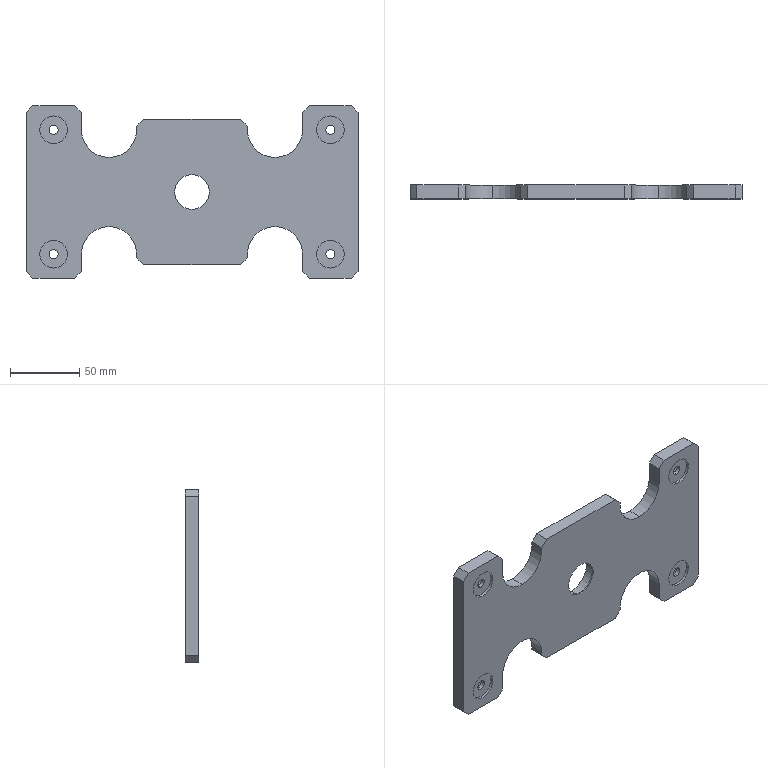Part | SolidWorks | features BaseBody 1 | 1 solid | 73 faces | box 240 x 10 x 125 mm | volume 216814 mm3 | plane 39 | cylinder 34 | commonest cylinder face diameters 6.6 x8 11 x8 20 x8 40 x6 25 x2 32 x2